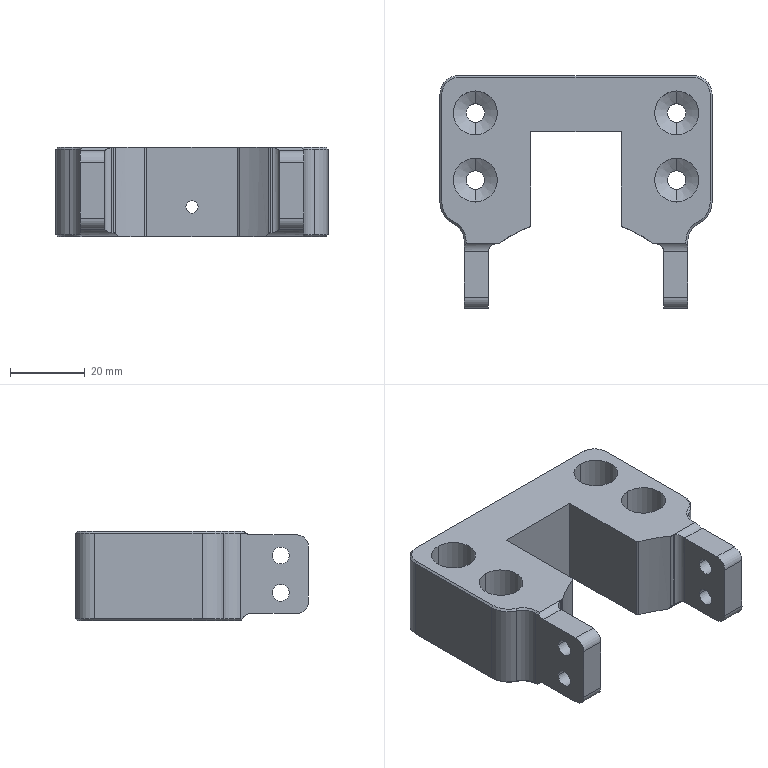NC program | NX | posted with a generic post | part box 73 x 62.4 x 24 mm
Lines 1 to 273 of 2496:
N10 G17 G21 G94 G90
(FLOOR_WALL_COPY , TOOL : D63)
N12 T01 M6
N14 G54
N16 G17 G0 G90 X-71. Y31.197 S6500 M3
N18 G43 Z30. H1
N20 Z8.
N22 G94 G1 Z5. F1250.
N24 X-68.
N26 X68.
N28 Y-6.
N30 X-68.
N32 X-71.
N34 Z8.
N36 G0 Z30.
N38 Y31.197
N40 Z7.
N42 G1 Z4.
N44 X-68.
N46 X68.
N48 Y-6.
N50 X-68.
N52 X-71.
N54 Z7.
N56 G0 Z30.
N58 Y31.197
N60 Z6.
N62 G1 Z3.
N64 X-68.
N66 X68.
N68 Y-6.
N70 X-68.
N72 X-71.
N74 Z6.
N76 G0 Z30.
N78 Y31.197
N80 Z5.
N82 G1 Z2.
N84 X-68.
N86 X68.
N88 Y-6.
N90 X-68.
N92 X-71.
N94 Z5.
N96 G0 Z30.
N98 Y31.197
N100 Z4.
N102 G1 Z1.
N104 X-68.
N106 X68.
N108 Y-6.
N110 X-68.
N112 X-71.
N114 Z4.
N116 G0 Z30.
N118 Y31.197
N120 Z3.
N122 G1 Z0.
N124 X-68.
N126 X68.
N128 Y-6.
N130 X-68.
N132 X-71.
N134 Z3.
N136 G0 Z30.
(FLOOR_WALL_COPY_COPY , TOOL : D63)
N138 G55
N140 Y31.197
N142 Z8.
N144 G1 Z5.
N146 X-68.
N148 X68.
N150 Y-6.
N152 X-68.
N154 X-71.
N156 Z8.
N158 G0 Z30.
N160 Y31.197
N162 Z7.
N164 G1 Z4.
N166 X-68.
N168 X68.
N170 Y-6.
N172 X-68.
N174 X-71.
N176 Z7.
N178 G0 Z30.
N180 Y31.197
N182 Z6.
N184 G1 Z3.
N186 X-68.
N188 X68.
N190 Y-6.
N192 X-68.
N194 X-71.
N196 Z6.
N198 G0 Z30.
N200 Y31.197
N202 Z5.
N204 G1 Z2.
N206 X-68.
N208 X68.
N210 Y-6.
N212 X-68.
N214 X-71.
N216 Z5.
N218 G0 Z30.
N220 Y31.197
N222 Z4.
N224 G1 Z1.
N226 X-68.
N228 X68.
N230 Y-6.
N232 X-68.
N234 X-71.
N236 Z4.
N238 G0 Z30.
N240 Y31.197
N242 Z3.
N244 G1 Z0.
N246 X-68.
N248 X68.
N250 Y-6.
N252 X-68.
N254 X-71.
N256 Z3.
N258 G0 Z30.
N260 M5
(FLOOR_WALL_1_1_COPY_COPY , TOOL : D10JING)
N262 T11 M6
N264 G54
N266 G17 G0 G90 X-17.36 Y-34.175 S7000 M3
N268 G43 Z30. H11
N270 Z0.5
N272 G94 G1 Z-1. F1250.
N274 X-17.634 Y-33.7
N276 G3 X-18.5 Y-33.2 R1.
N278 G1 X-35.
N280 Y-29.152
N282 X-18.5
N284 Y-25.104
N286 X-35.
N288 Y-21.056
N290 X-18.5
N292 G2 X-17.634 Y-21.556 R1.
N294 G1 X-17. Y-22.654
N296 Z0.5
N298 G0 Z30.
N300 X-17.36 Y-34.175
N302 Z-0.5
N304 G1 Z-2.
N306 X-17.634 Y-33.7
N308 G3 X-18.5 Y-33.2 R1.
N310 G1 X-35.
N312 Y-29.152
N314 X-18.5
N316 Y-25.104
N318 X-35.
N320 Y-21.056
N322 X-18.5
N324 G2 X-17.634 Y-21.556 R1.
N326 G1 X-17. Y-22.654
N328 Z-0.5
N330 G0 Z30.
N332 X36.14 Y-34.175
N334 Z0.5
N336 G1 Z-1.
N338 X35.866 Y-33.7
N340 G3 X35. Y-33.2 R1.
N342 G1 X18.5
N344 Y-29.152
N346 X35.
N348 Y-25.104
N350 X18.5
N352 Y-21.056
N354 X35.
N356 G2 X35.866 Y-21.556 R1.
N358 G1 X36.5 Y-22.654
N360 Z0.5
N362 G0 Z30.
N364 X36.14 Y-34.175
N366 Z-0.5
N368 G1 Z-2.
N370 X35.866 Y-33.7
N372 G3 X35. Y-33.2 R1.
N374 G1 X18.5
N376 Y-29.152
N378 X35.
N380 Y-25.104
N382 X18.5
N384 Y-21.056
N386 X35.
N388 G2 X35.866 Y-21.556 R1.
N390 G1 X36.5 Y-22.654
N392 Z-0.5
N394 G0 Z30.
(FLOOR_WALL_1_1_COPY_COPY_COPY , TOOL : D10JING)
N396 G55
N398 X-17.36 Y-34.175
N400 Z0.5
N402 G1 Z-1.
N404 X-17.634 Y-33.7
N406 G3 X-18.5 Y-33.2 R1.
N408 G1 X-35.
N410 Y-29.152
N412 X-18.5
N414 Y-25.104
N416 X-35.
N418 Y-21.056
N420 X-18.5
N422 G2 X-17.634 Y-21.556 R1.
N424 G1 X-17. Y-22.654
N426 Z0.5
N428 G0 Z30.
N430 X-17.36 Y-34.175
N432 Z-0.5
N434 G1 Z-2.
N436 X-17.634 Y-33.7
N438 G3 X-18.5 Y-33.2 R1.
N440 G1 X-35.
N442 Y-29.152
N444 X-18.5
N446 Y-25.104
N448 X-35.
N450 Y-21.056
N452 X-18.5
N454 G2 X-17.634 Y-21.556 R1.
N456 G1 X-17. Y-22.654
N458 Z-0.5
N460 G0 Z30.
N462 X36.14 Y-34.175
N464 Z0.5
N466 G1 Z-1.
N468 X35.866 Y-33.7
N470 G3 X35. Y-33.2 R1.
N472 G1 X18.5
N474 Y-29.152
N476 X35.
N478 Y-25.104
N480 X18.5
N482 Y-21.056
N484 X35.
N486 G2 X35.866 Y-21.556 R1.
N488 G1 X36.5 Y-22.654
N490 Z0.5
N492 G0 Z30.
N494 X36.14 Y-34.175
N496 Z-0.5
N498 G1 Z-2.
N500 X35.866 Y-33.7
N502 G3 X35. Y-33.2 R1.
N504 G1 X18.5
N506 Y-29.152
N508 X35.
N510 Y-25.104
N512 X18.5
N514 Y-21.056
N516 X35.
N518 G2 X35.866 Y-21.556 R1.
N520 G1 X36.5 Y-22.654
N522 Z-0.5
N524 G0 Z30.
N526 M5